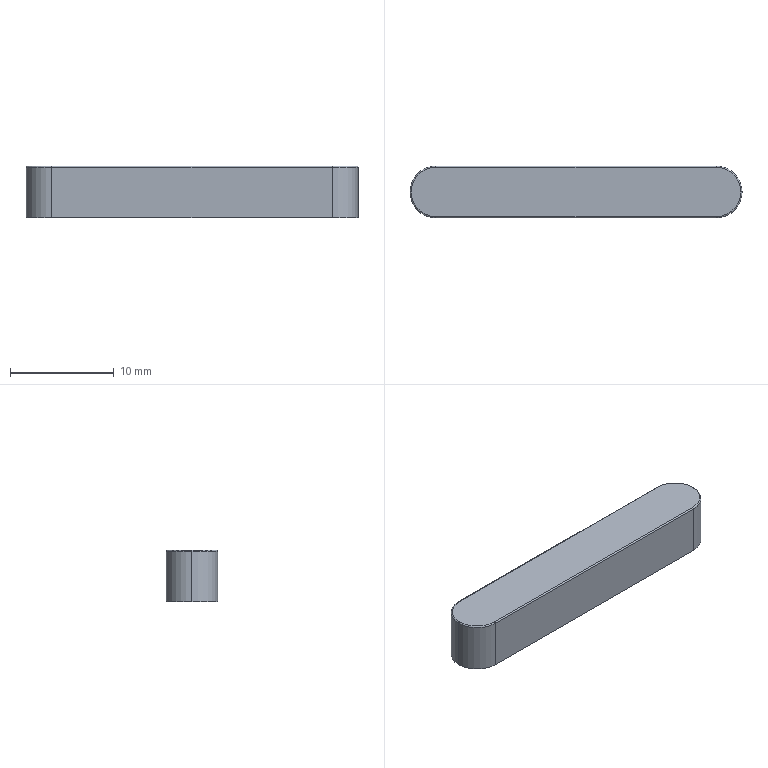Part | NX | features BLEND 2, DATUM_CSYS 2, EXTRUDE 1, SKETCH 1 | 1 solid | 14 faces | box 32 x 5 x 5 mm | volume 772.96 mm3 | cylinder 6 | plane 4 | torus 4 | commonest cylinder face diameters 5 x4 0.24 x2
STEP:
#1=CARTESIAN_POINT('',(13.5,-2.5,0.));
#2=VERTEX_POINT('',#1);
#3=CARTESIAN_POINT('',(13.5,-2.5,4.88));
#4=VERTEX_POINT('',#3);
#5=CARTESIAN_POINT('',(13.5,-2.5,5.));
#6=DIRECTION('',(0.,0.,-1.));
#7=VECTOR('',#6,1000.);
#8=LINE('',#5,#7);
#9=EDGE_CURVE('',#2,#4,#8,.F.);
#10=ORIENTED_EDGE('',*,*,#9,.T.);
#11=CARTESIAN_POINT('',(-13.5,-2.5,4.88));
#12=VERTEX_POINT('',#11);
#13=CARTESIAN_POINT('',(-13.5,-2.5,4.88));
#14=DIRECTION('',(1.,0.,0.));
#15=VECTOR('',#14,1000.);
#16=LINE('',#13,#15);
#17=EDGE_CURVE('',#4,#12,#16,.F.);
#18=ORIENTED_EDGE('',*,*,#17,.T.);
#19=CARTESIAN_POINT('',(-13.5,-2.5,0.));
#20=VERTEX_POINT('',#19);
#21=CARTESIAN_POINT('',(-13.5,-2.5,5.));
#22=DIRECTION('',(0.,0.,-1.));
#23=VECTOR('',#22,1000.);
#24=LINE('',#21,#23);
#25=EDGE_CURVE('',#12,#20,#24,.T.);
#26=ORIENTED_EDGE('',*,*,#25,.T.);
#27=CARTESIAN_POINT('',(-16.,-2.5,0.));
#28=DIRECTION('',(1.,0.,0.));
#29=VECTOR('',#28,1000.);
#30=LINE('',#27,#29);
#31=EDGE_CURVE('',#20,#2,#30,.T.);
#32=ORIENTED_EDGE('',*,*,#31,.T.);
#33=EDGE_LOOP('',(#10,#18,#26,#32));
#34=FACE_BOUND('',#33,.T.);
#35=CARTESIAN_POINT('',(-16.,-2.5,5.));
#36=DIRECTION('',(0.,1.,0.));
#37=DIRECTION('',(0.,0.,1.));
#38=AXIS2_PLACEMENT_3D('',#35,#36,#37);
#39=PLANE('',#38);
#40=ADVANCED_FACE('',(#34),#39,.F.);
#41=CARTESIAN_POINT('',(-13.5,2.5,0.));
#42=VERTEX_POINT('',#41);
#43=CARTESIAN_POINT('',(-13.5,2.5,4.88));
#44=VERTEX_POINT('',#43);
#45=CARTESIAN_POINT('',(-13.5,2.5,5.));
#46=DIRECTION('',(0.,0.,-1.));
#47=VECTOR('',#46,1000.);
#48=LINE('',#45,#47);
#49=EDGE_CURVE('',#42,#44,#48,.F.);
#50=ORIENTED_EDGE('',*,*,#49,.T.);
#51=CARTESIAN_POINT('',(13.5,2.5,4.88));
#52=VERTEX_POINT('',#51);
#53=CARTESIAN_POINT('',(13.5,2.5,4.88));
#54=DIRECTION('',(-1.,0.,0.));
#55=VECTOR('',#54,1000.);
#56=LINE('',#53,#55);
#57=EDGE_CURVE('',#44,#52,#56,.F.);
#58=ORIENTED_EDGE('',*,*,#57,.T.);
#59=CARTESIAN_POINT('',(13.5,2.5,0.));
#60=VERTEX_POINT('',#59);
#61=CARTESIAN_POINT('',(13.5,2.5,5.));
#62=DIRECTION('',(0.,0.,-1.));
#63=VECTOR('',#62,1000.);
#64=LINE('',#61,#63);
#65=EDGE_CURVE('',#52,#60,#64,.T.);
#66=ORIENTED_EDGE('',*,*,#65,.T.);
#67=CARTESIAN_POINT('',(16.,2.5,0.));
#68=DIRECTION('',(-1.,0.,0.));
#69=VECTOR('',#68,1000.);
#70=LINE('',#67,#69);
#71=EDGE_CURVE('',#60,#42,#70,.T.);
#72=ORIENTED_EDGE('',*,*,#71,.T.);
#73=EDGE_LOOP('',(#50,#58,#66,#72));
#74=FACE_BOUND('',#73,.T.);
#75=CARTESIAN_POINT('',(16.,2.5,5.));
#76=DIRECTION('',(0.,-1.,0.));
#77=DIRECTION('',(0.,0.,-1.));
#78=AXIS2_PLACEMENT_3D('',#75,#76,#77);
#79=PLANE('',#78);
#80=ADVANCED_FACE('',(#74),#79,.F.);
#81=CARTESIAN_POINT('',(-13.5,2.38,5.));
#82=VERTEX_POINT('',#81);
#83=CARTESIAN_POINT('',(-15.88,0.,5.));
#84=VERTEX_POINT('',#83);
#85=CARTESIAN_POINT('',(-13.5,0.,5.));
#86=DIRECTION('',(0.,0.,1.));
#87=DIRECTION('',(1.,0.,0.));
#88=AXIS2_PLACEMENT_3D('',#85,#86,#87);
#89=CIRCLE('',#88,2.38);
#90=EDGE_CURVE('',#82,#84,#89,.T.);
#91=ORIENTED_EDGE('',*,*,#90,.T.);
#92=CARTESIAN_POINT('',(-13.5,-2.38,5.));
#93=VERTEX_POINT('',#92);
#94=CARTESIAN_POINT('',(-13.5,0.,5.));
#95=DIRECTION('',(0.,0.,1.));
#96=DIRECTION('',(1.,0.,0.));
#97=AXIS2_PLACEMENT_3D('',#94,#95,#96);
#98=CIRCLE('',#97,2.38);
#99=EDGE_CURVE('',#84,#93,#98,.T.);
#100=ORIENTED_EDGE('',*,*,#99,.T.);
#101=CARTESIAN_POINT('',(13.5,-2.38,5.));
#102=VERTEX_POINT('',#101);
#103=CARTESIAN_POINT('',(13.5,-2.38,5.));
#104=DIRECTION('',(1.,0.,0.));
#105=VECTOR('',#104,1000.);
#106=LINE('',#103,#105);
#107=EDGE_CURVE('',#93,#102,#106,.T.);
#108=ORIENTED_EDGE('',*,*,#107,.T.);
#109=CARTESIAN_POINT('',(15.88,0.,5.));
#110=VERTEX_POINT('',#109);
#111=CARTESIAN_POINT('',(13.5,0.,5.));
#112=DIRECTION('',(0.,0.,1.));
#113=DIRECTION('',(1.,0.,0.));
#114=AXIS2_PLACEMENT_3D('',#111,#112,#113);
#115=CIRCLE('',#114,2.38);
#116=EDGE_CURVE('',#102,#110,#115,.T.);
#117=ORIENTED_EDGE('',*,*,#116,.T.);
#118=CARTESIAN_POINT('',(13.5,2.38,5.));
#119=VERTEX_POINT('',#118);
#120=CARTESIAN_POINT('',(13.5,0.,5.));
#121=DIRECTION('',(0.,0.,1.));
#122=DIRECTION('',(1.,0.,0.));
#123=AXIS2_PLACEMENT_3D('',#120,#121,#122);
#124=CIRCLE('',#123,2.38);
#125=EDGE_CURVE('',#110,#119,#124,.T.);
#126=ORIENTED_EDGE('',*,*,#125,.T.);
#127=CARTESIAN_POINT('',(-13.5,2.38,5.));
#128=DIRECTION('',(-1.,0.,0.));
#129=VECTOR('',#128,1000.);
#130=LINE('',#127,#129);
#131=EDGE_CURVE('',#119,#82,#130,.T.);
#132=ORIENTED_EDGE('',*,*,#131,.T.);
#133=EDGE_LOOP('',(#91,#100,#108,#117,#126,#132));
#134=FACE_BOUND('',#133,.T.);
#135=CARTESIAN_POINT('',(0.,0.,5.));
#136=DIRECTION('',(0.,0.,1.));
#137=DIRECTION('',(1.,0.,0.));
#138=AXIS2_PLACEMENT_3D('',#135,#136,#137);
#139=PLANE('',#138);
#140=ADVANCED_FACE('',(#134),#139,.T.);
#141=CARTESIAN_POINT('',(-16.,0.,0.));
#142=VERTEX_POINT('',#141);
#143=CARTESIAN_POINT('',(-13.5,0.,0.));
#144=DIRECTION('',(0.,0.,1.));
#145=DIRECTION('',(1.,0.,0.));
#146=AXIS2_PLACEMENT_3D('',#143,#144,#145);
#147=CIRCLE('',#146,2.5);
#148=EDGE_CURVE('',#20,#142,#147,.F.);
#149=ORIENTED_EDGE('',*,*,#148,.T.);
#150=CARTESIAN_POINT('',(-13.5,0.,0.));
#151=DIRECTION('',(0.,0.,1.));
#152=DIRECTION('',(1.,0.,0.));
#153=AXIS2_PLACEMENT_3D('',#150,#151,#152);
#154=CIRCLE('',#153,2.5);
#155=EDGE_CURVE('',#142,#42,#154,.F.);
#156=ORIENTED_EDGE('',*,*,#155,.T.);
#157=ORIENTED_EDGE('',*,*,#71,.F.);
#158=CARTESIAN_POINT('',(16.,0.,0.));
#159=VERTEX_POINT('',#158);
#160=CARTESIAN_POINT('',(13.5,0.,0.));
#161=DIRECTION('',(0.,0.,1.));
#162=DIRECTION('',(1.,0.,0.));
#163=AXIS2_PLACEMENT_3D('',#160,#161,#162);
#164=CIRCLE('',#163,2.5);
#165=EDGE_CURVE('',#60,#159,#164,.F.);
#166=ORIENTED_EDGE('',*,*,#165,.T.);
#167=CARTESIAN_POINT('',(13.5,0.,0.));
#168=DIRECTION('',(0.,0.,1.));
#169=DIRECTION('',(1.,0.,0.));
#170=AXIS2_PLACEMENT_3D('',#167,#168,#169);
#171=CIRCLE('',#170,2.5);
#172=EDGE_CURVE('',#159,#2,#171,.F.);
#173=ORIENTED_EDGE('',*,*,#172,.T.);
#174=ORIENTED_EDGE('',*,*,#31,.F.);
#175=EDGE_LOOP('',(#149,#156,#157,#166,#173,#174));
#176=FACE_BOUND('',#175,.T.);
#177=CARTESIAN_POINT('',(0.,0.,0.));
#178=DIRECTION('',(0.,0.,1.));
#179=DIRECTION('',(1.,0.,0.));
#180=AXIS2_PLACEMENT_3D('',#177,#178,#179);
#181=PLANE('',#180);
#182=ADVANCED_FACE('',(#176),#181,.F.);
#183=ORIENTED_EDGE('',*,*,#25,.F.);
#184=CARTESIAN_POINT('',(-16.,0.,4.88));
#185=VERTEX_POINT('',#184);
#186=CARTESIAN_POINT('',(-13.5,0.,4.88));
#187=DIRECTION('',(0.,0.,1.));
#188=DIRECTION('',(1.,0.,0.));
#189=AXIS2_PLACEMENT_3D('',#186,#187,#188);
#190=CIRCLE('',#189,2.5);
#191=EDGE_CURVE('',#12,#185,#190,.F.);
#192=ORIENTED_EDGE('',*,*,#191,.T.);
#193=CARTESIAN_POINT('',(-16.,0.,5.));
#194=DIRECTION('',(0.,0.,-1.));
#195=VECTOR('',#194,1000.);
#196=LINE('',#193,#195);
#197=EDGE_CURVE('',#142,#185,#196,.F.);
#198=ORIENTED_EDGE('',*,*,#197,.F.);
#199=ORIENTED_EDGE('',*,*,#148,.F.);
#200=EDGE_LOOP('',(#183,#192,#198,#199));
#201=FACE_BOUND('',#200,.T.);
#202=CARTESIAN_POINT('',(-13.5,0.,5.));
#203=DIRECTION('',(0.,0.,-1.));
#204=DIRECTION('',(-1.,0.,0.));
#205=AXIS2_PLACEMENT_3D('',#202,#203,#204);
#206=CYLINDRICAL_SURFACE('',#205,2.5);
#207=ADVANCED_FACE('',(#201),#206,.T.);
#208=ORIENTED_EDGE('',*,*,#197,.T.);
#209=CARTESIAN_POINT('',(-13.5,0.,4.88));
#210=DIRECTION('',(0.,0.,1.));
#211=DIRECTION('',(1.,0.,0.));
#212=AXIS2_PLACEMENT_3D('',#209,#210,#211);
#213=CIRCLE('',#212,2.5);
#214=EDGE_CURVE('',#185,#44,#213,.F.);
#215=ORIENTED_EDGE('',*,*,#214,.T.);
#216=ORIENTED_EDGE('',*,*,#49,.F.);
#217=ORIENTED_EDGE('',*,*,#155,.F.);
#218=EDGE_LOOP('',(#208,#215,#216,#217));
#219=FACE_BOUND('',#218,.T.);
#220=CARTESIAN_POINT('',(-13.5,0.,5.));
#221=DIRECTION('',(0.,0.,-1.));
#222=DIRECTION('',(-1.,0.,0.));
#223=AXIS2_PLACEMENT_3D('',#220,#221,#222);
#224=CYLINDRICAL_SURFACE('',#223,2.5);
#225=ADVANCED_FACE('',(#219),#224,.T.);
#226=CARTESIAN_POINT('',(16.,0.,4.88));
#227=VERTEX_POINT('',#226);
#228=CARTESIAN_POINT('',(16.,0.,5.));
#229=DIRECTION('',(0.,0.,-1.));
#230=VECTOR('',#229,1000.);
#231=LINE('',#228,#230);
#232=EDGE_CURVE('',#227,#159,#231,.T.);
#233=ORIENTED_EDGE('',*,*,#232,.F.);
#234=CARTESIAN_POINT('',(13.5,0.,4.88));
#235=DIRECTION('',(0.,0.,1.));
#236=DIRECTION('',(1.,0.,0.));
#237=AXIS2_PLACEMENT_3D('',#234,#235,#236);
#238=CIRCLE('',#237,2.5);
#239=EDGE_CURVE('',#227,#4,#238,.F.);
#240=ORIENTED_EDGE('',*,*,#239,.T.);
#241=ORIENTED_EDGE('',*,*,#9,.F.);
#242=ORIENTED_EDGE('',*,*,#172,.F.);
#243=EDGE_LOOP('',(#233,#240,#241,#242));
#244=FACE_BOUND('',#243,.T.);
#245=CARTESIAN_POINT('',(13.5,0.,5.));
#246=DIRECTION('',(0.,0.,-1.));
#247=DIRECTION('',(-1.,0.,0.));
#248=AXIS2_PLACEMENT_3D('',#245,#246,#247);
#249=CYLINDRICAL_SURFACE('',#248,2.5);
#250=ADVANCED_FACE('',(#244),#249,.T.);
#251=ORIENTED_EDGE('',*,*,#65,.F.);
#252=CARTESIAN_POINT('',(13.5,0.,4.88));
#253=DIRECTION('',(0.,0.,1.));
#254=DIRECTION('',(1.,0.,0.));
#255=AXIS2_PLACEMENT_3D('',#252,#253,#254);
#256=CIRCLE('',#255,2.5);
#257=EDGE_CURVE('',#52,#227,#256,.F.);
#258=ORIENTED_EDGE('',*,*,#257,.T.);
#259=ORIENTED_EDGE('',*,*,#232,.T.);
#260=ORIENTED_EDGE('',*,*,#165,.F.);
#261=EDGE_LOOP('',(#251,#258,#259,#260));
#262=FACE_BOUND('',#261,.T.);
#263=CARTESIAN_POINT('',(13.5,0.,5.));
#264=DIRECTION('',(0.,0.,-1.));
#265=DIRECTION('',(-1.,0.,0.));
#266=AXIS2_PLACEMENT_3D('',#263,#264,#265);
#267=CYLINDRICAL_SURFACE('',#266,2.5);
#268=ADVANCED_FACE('',(#262),#267,.T.);
#269=CARTESIAN_POINT('',(15.88,0.,4.88));
#270=DIRECTION('',(0.,-1.,0.));
#271=DIRECTION('',(1.,0.,0.));
#272=AXIS2_PLACEMENT_3D('',#269,#270,#271);
#273=CIRCLE('',#272,0.12);
#274=EDGE_CURVE('',#227,#110,#273,.T.);
#275=ORIENTED_EDGE('',*,*,#274,.F.);
#276=ORIENTED_EDGE('',*,*,#257,.F.);
#277=CARTESIAN_POINT('',(13.5,2.38,4.88));
#278=DIRECTION('',(-1.,0.,0.));
#279=DIRECTION('',(0.,0.,1.));
#280=AXIS2_PLACEMENT_3D('',#277,#278,#279);
#281=CIRCLE('',#280,0.12);
#282=EDGE_CURVE('',#119,#52,#281,.T.);
#283=ORIENTED_EDGE('',*,*,#282,.F.);
#284=ORIENTED_EDGE('',*,*,#125,.F.);
#285=EDGE_LOOP('',(#275,#276,#283,#284));
#286=FACE_BOUND('',#285,.T.);
#287=CARTESIAN_POINT('',(13.5,0.,4.88));
#288=DIRECTION('',(0.,0.,1.));
#289=DIRECTION('',(1.,0.,0.));
#290=AXIS2_PLACEMENT_3D('',#287,#288,#289);
#291=TOROIDAL_SURFACE('',#290,2.38,0.12);
#292=ADVANCED_FACE('',(#286),#291,.T.);
#293=ORIENTED_EDGE('',*,*,#282,.T.);
#294=ORIENTED_EDGE('',*,*,#57,.F.);
#295=CARTESIAN_POINT('',(-13.5,2.38,4.88));
#296=DIRECTION('',(-1.,0.,0.));
#297=DIRECTION('',(0.,0.,1.));
#298=AXIS2_PLACEMENT_3D('',#295,#296,#297);
#299=CIRCLE('',#298,0.12);
#300=EDGE_CURVE('',#82,#44,#299,.T.);
#301=ORIENTED_EDGE('',*,*,#300,.F.);
#302=ORIENTED_EDGE('',*,*,#131,.F.);
#303=EDGE_LOOP('',(#293,#294,#301,#302));
#304=FACE_BOUND('',#303,.T.);
#305=CARTESIAN_POINT('',(0.,2.38,4.88));
#306=DIRECTION('',(1.,0.,0.));
#307=DIRECTION('',(0.,0.,-1.));
#308=AXIS2_PLACEMENT_3D('',#305,#306,#307);
#309=CYLINDRICAL_SURFACE('',#308,0.12);
#310=ADVANCED_FACE('',(#304),#309,.T.);
#311=ORIENTED_EDGE('',*,*,#274,.T.);
#312=ORIENTED_EDGE('',*,*,#116,.F.);
#313=CARTESIAN_POINT('',(13.5,-2.38,4.88));
#314=DIRECTION('',(-1.,0.,0.));
#315=DIRECTION('',(0.,0.,1.));
#316=AXIS2_PLACEMENT_3D('',#313,#314,#315);
#317=CIRCLE('',#316,0.12);
#318=EDGE_CURVE('',#4,#102,#317,.T.);
#319=ORIENTED_EDGE('',*,*,#318,.F.);
#320=ORIENTED_EDGE('',*,*,#239,.F.);
#321=EDGE_LOOP('',(#311,#312,#319,#320));
#322=FACE_BOUND('',#321,.T.);
#323=CARTESIAN_POINT('',(13.5,0.,4.88));
#324=DIRECTION('',(0.,0.,1.));
#325=DIRECTION('',(1.,0.,0.));
#326=AXIS2_PLACEMENT_3D('',#323,#324,#325);
#327=TOROIDAL_SURFACE('',#326,2.38,0.12);
#328=ADVANCED_FACE('',(#322),#327,.T.);
#329=ORIENTED_EDGE('',*,*,#300,.T.);
#330=ORIENTED_EDGE('',*,*,#214,.F.);
#331=CARTESIAN_POINT('',(-15.88,0.,4.88));
#332=DIRECTION('',(0.,-1.,0.));
#333=DIRECTION('',(0.,0.,-1.));
#334=AXIS2_PLACEMENT_3D('',#331,#332,#333);
#335=CIRCLE('',#334,0.12);
#336=EDGE_CURVE('',#84,#185,#335,.T.);
#337=ORIENTED_EDGE('',*,*,#336,.F.);
#338=ORIENTED_EDGE('',*,*,#90,.F.);
#339=EDGE_LOOP('',(#329,#330,#337,#338));
#340=FACE_BOUND('',#339,.T.);
#341=CARTESIAN_POINT('',(-13.5,0.,4.88));
#342=DIRECTION('',(0.,0.,1.));
#343=DIRECTION('',(1.,0.,0.));
#344=AXIS2_PLACEMENT_3D('',#341,#342,#343);
#345=TOROIDAL_SURFACE('',#344,2.38,0.12);
#346=ADVANCED_FACE('',(#340),#345,.T.);
#347=ORIENTED_EDGE('',*,*,#318,.T.);
#348=ORIENTED_EDGE('',*,*,#107,.F.);
#349=CARTESIAN_POINT('',(-13.5,-2.38,4.88));
#350=DIRECTION('',(-1.,0.,0.));
#351=DIRECTION('',(0.,0.,1.));
#352=AXIS2_PLACEMENT_3D('',#349,#350,#351);
#353=CIRCLE('',#352,0.12);
#354=EDGE_CURVE('',#12,#93,#353,.T.);
#355=ORIENTED_EDGE('',*,*,#354,.F.);
#356=ORIENTED_EDGE('',*,*,#17,.F.);
#357=EDGE_LOOP('',(#347,#348,#355,#356));
#358=FACE_BOUND('',#357,.T.);
#359=CARTESIAN_POINT('',(0.,-2.38,4.88));
#360=DIRECTION('',(-1.,0.,0.));
#361=DIRECTION('',(0.,0.,1.));
#362=AXIS2_PLACEMENT_3D('',#359,#360,#361);
#363=CYLINDRICAL_SURFACE('',#362,0.12);
#364=ADVANCED_FACE('',(#358),#363,.T.);
#365=ORIENTED_EDGE('',*,*,#336,.T.);
#366=ORIENTED_EDGE('',*,*,#191,.F.);
#367=ORIENTED_EDGE('',*,*,#354,.T.);
#368=ORIENTED_EDGE('',*,*,#99,.F.);
#369=EDGE_LOOP('',(#365,#366,#367,#368));
#370=FACE_BOUND('',#369,.T.);
#371=CARTESIAN_POINT('',(-13.5,0.,4.88));
#372=DIRECTION('',(0.,0.,1.));
#373=DIRECTION('',(1.,0.,0.));
#374=AXIS2_PLACEMENT_3D('',#371,#372,#373);
#375=TOROIDAL_SURFACE('',#374,2.38,0.12);
#376=ADVANCED_FACE('',(#370),#375,.T.);
#377=CLOSED_SHELL('',(#40,#80,#140,#182,#207,#225,#250,#268,#292,#310,#328,#346,#364,#376));
#378=MANIFOLD_SOLID_BREP('',#377);
#379=(LENGTH_UNIT()NAMED_UNIT(*)SI_UNIT(.MILLI.,.METRE.));
#380=UNCERTAINTY_MEASURE_WITH_UNIT(LENGTH_MEASURE(0.00001),#379,'','');
#381=(NAMED_UNIT(*)PLANE_ANGLE_UNIT()SI_UNIT($,.RADIAN.));
#382=(NAMED_UNIT(*)SI_UNIT($,.STERADIAN.)SOLID_ANGLE_UNIT());
#383=(GEOMETRIC_REPRESENTATION_CONTEXT(3)GLOBAL_UNCERTAINTY_ASSIGNED_CONTEXT((#380))GLOBAL_UNIT_ASSIGNED_CONTEXT((#379,#381,#382))REPRESENTATION_CONTEXT('',''));
#384=ADVANCED_BREP_SHAPE_REPRESENTATION('',(#378),#383);